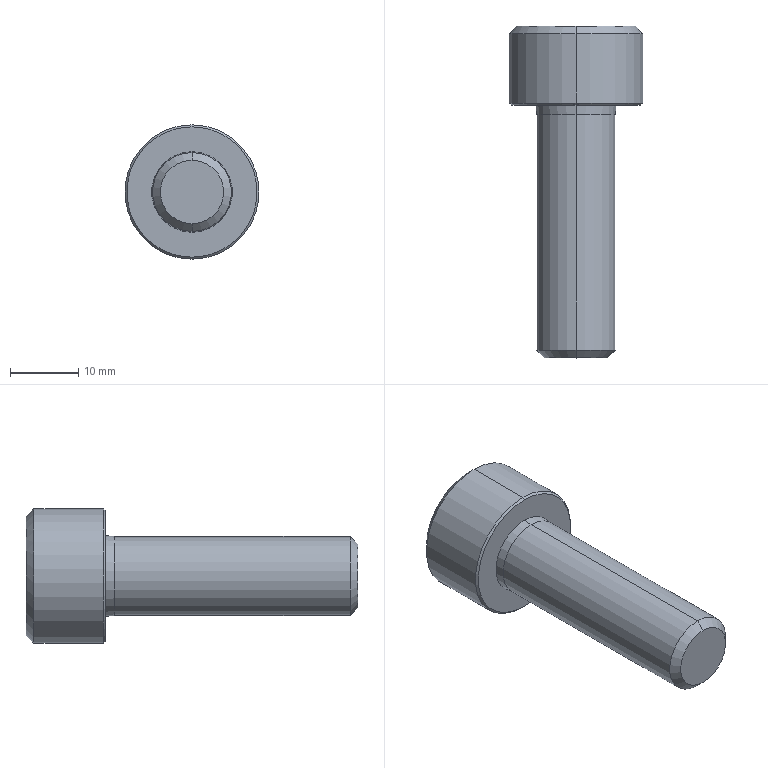Part | SolidWorks | features BaseBody 1 | 1 solid | 35 faces | box 19.615 x 48.462 x 19.615 mm | volume 6797 mm3 | cone 16 | plane 15 | cylinder 4 | commonest cylinder face diameters 11.538 x2 19.615 x2
STEP:
#1=CARTESIAN_POINT('',(-30.446,251.324,298.077));
#2=VERTEX_POINT('',#1);
#3=CARTESIAN_POINT('',(-30.446,251.324,286.538));
#4=VERTEX_POINT('',#3);
#5=CARTESIAN_POINT('',(-30.446,251.324,292.308));
#6=DIRECTION('',(0.,1.,0.));
#7=DIRECTION('',(0.,0.,1.));
#8=AXIS2_PLACEMENT_3D('',#5,#6,#7);
#9=CIRCLE('',#8,5.769);
#10=EDGE_CURVE('',#2,#4,#9,.T.);
#11=ORIENTED_EDGE('',*,*,#10,.T.);
#12=CARTESIAN_POINT('',(-30.446,285.731,286.538));
#13=VERTEX_POINT('',#12);
#14=CARTESIAN_POINT('',(-30.446,250.192,286.538));
#15=DIRECTION('',(0.,1.,0.));
#16=VECTOR('',#15,1000.);
#17=LINE('',#14,#16);
#18=EDGE_CURVE('',#4,#13,#17,.T.);
#19=ORIENTED_EDGE('',*,*,#18,.T.);
#20=CARTESIAN_POINT('',(-30.446,285.731,298.077));
#21=VERTEX_POINT('',#20);
#22=CARTESIAN_POINT('',(-30.446,285.731,292.308));
#23=DIRECTION('',(0.,-1.,0.));
#24=DIRECTION('',(0.,0.,1.));
#25=AXIS2_PLACEMENT_3D('',#22,#23,#24);
#26=CIRCLE('',#25,5.769);
#27=EDGE_CURVE('',#13,#21,#26,.T.);
#28=ORIENTED_EDGE('',*,*,#27,.T.);
#29=CARTESIAN_POINT('',(-30.446,250.192,298.077));
#30=DIRECTION('',(0.,1.,0.));
#31=VECTOR('',#30,1000.);
#32=LINE('',#29,#31);
#33=EDGE_CURVE('',#2,#21,#32,.T.);
#34=ORIENTED_EDGE('',*,*,#33,.F.);
#35=EDGE_LOOP('',(#11,#19,#28,#34));
#36=FACE_OUTER_BOUND('',#35,.T.);
#37=CARTESIAN_POINT('',(-30.446,250.192,292.308));
#38=DIRECTION('',(0.,1.,0.));
#39=DIRECTION('',(0.,0.,1.));
#40=AXIS2_PLACEMENT_3D('',#37,#38,#39);
#41=CYLINDRICAL_SURFACE('',#40,5.769);
#42=ADVANCED_FACE('',(#36),#41,.T.);
#43=CARTESIAN_POINT('',(-30.446,250.192,296.945));
#44=VERTEX_POINT('',#43);
#45=CARTESIAN_POINT('',(-30.446,250.192,287.67));
#46=VERTEX_POINT('',#45);
#47=CARTESIAN_POINT('',(-30.446,250.192,292.308));
#48=DIRECTION('',(0.,1.,0.));
#49=DIRECTION('',(0.,0.,1.));
#50=AXIS2_PLACEMENT_3D('',#47,#48,#49);
#51=CIRCLE('',#50,4.637);
#52=EDGE_CURVE('',#44,#46,#51,.T.);
#53=ORIENTED_EDGE('',*,*,#52,.T.);
#54=CARTESIAN_POINT('',(-30.446,251.324,286.538));
#55=DIRECTION('',(0.,0.7071,-0.7071));
#56=VECTOR('',#55,1000.);
#57=LINE('',#54,#56);
#58=EDGE_CURVE('',#46,#4,#57,.T.);
#59=ORIENTED_EDGE('',*,*,#58,.T.);
#60=ORIENTED_EDGE('',*,*,#10,.F.);
#61=CARTESIAN_POINT('',(-30.446,251.324,298.077));
#62=DIRECTION('',(0.,0.7071,0.7071));
#63=VECTOR('',#62,1000.);
#64=LINE('',#61,#63);
#65=EDGE_CURVE('',#44,#2,#64,.T.);
#66=ORIENTED_EDGE('',*,*,#65,.F.);
#67=EDGE_LOOP('',(#53,#59,#60,#66));
#68=FACE_OUTER_BOUND('',#67,.T.);
#69=CARTESIAN_POINT('',(-30.446,251.324,292.308));
#70=DIRECTION('',(0.,1.,0.));
#71=DIRECTION('',(0.,0.,1.));
#72=AXIS2_PLACEMENT_3D('',#69,#70,#71);
#73=CONICAL_SURFACE('',#72,5.769,0.7854);
#74=ADVANCED_FACE('',(#68),#73,.T.);
#75=ORIENTED_EDGE('',*,*,#27,.F.);
#76=CARTESIAN_POINT('',(-30.446,287.115,286.423));
#77=VERTEX_POINT('',#76);
#78=CARTESIAN_POINT('',(-30.446,287.115,286.423));
#79=DIRECTION('',(0.,0.9965,-0.08305));
#80=VECTOR('',#79,1000.);
#81=LINE('',#78,#80);
#82=EDGE_CURVE('',#13,#77,#81,.T.);
#83=ORIENTED_EDGE('',*,*,#82,.T.);
#84=CARTESIAN_POINT('',(-30.446,287.115,298.192));
#85=VERTEX_POINT('',#84);
#86=CARTESIAN_POINT('',(-30.446,287.115,292.308));
#87=DIRECTION('',(0.,-1.,0.));
#88=DIRECTION('',(0.,0.,1.));
#89=AXIS2_PLACEMENT_3D('',#86,#87,#88);
#90=CIRCLE('',#89,5.885);
#91=EDGE_CURVE('',#77,#85,#90,.T.);
#92=ORIENTED_EDGE('',*,*,#91,.T.);
#93=CARTESIAN_POINT('',(-30.446,287.115,298.192));
#94=DIRECTION('',(0.,0.9965,0.08305));
#95=VECTOR('',#94,1000.);
#96=LINE('',#93,#95);
#97=EDGE_CURVE('',#21,#85,#96,.T.);
#98=ORIENTED_EDGE('',*,*,#97,.F.);
#99=EDGE_LOOP('',(#75,#83,#92,#98));
#100=FACE_OUTER_BOUND('',#99,.T.);
#101=CARTESIAN_POINT('',(-30.446,287.115,292.308));
#102=DIRECTION('',(0.,1.,0.));
#103=DIRECTION('',(0.,0.,1.));
#104=AXIS2_PLACEMENT_3D('',#101,#102,#103);
#105=CONICAL_SURFACE('',#104,5.885,0.08314);
#106=ADVANCED_FACE('',(#100),#105,.T.);
#107=CARTESIAN_POINT('',(-30.446,287.115,301.827));
#108=VERTEX_POINT('',#107);
#109=CARTESIAN_POINT('',(-30.446,287.115,282.788));
#110=VERTEX_POINT('',#109);
#111=CARTESIAN_POINT('',(-30.446,287.115,292.308));
#112=DIRECTION('',(0.,1.,0.));
#113=DIRECTION('',(0.,0.,1.));
#114=AXIS2_PLACEMENT_3D('',#111,#112,#113);
#115=CIRCLE('',#114,9.519);
#116=EDGE_CURVE('',#108,#110,#115,.T.);
#117=ORIENTED_EDGE('',*,*,#116,.T.);
#118=CARTESIAN_POINT('',(-30.446,287.404,282.5));
#119=VERTEX_POINT('',#118);
#120=CARTESIAN_POINT('',(-30.446,287.404,282.5));
#121=DIRECTION('',(0.,0.7071,-0.7071));
#122=VECTOR('',#121,1000.);
#123=LINE('',#120,#122);
#124=EDGE_CURVE('',#110,#119,#123,.T.);
#125=ORIENTED_EDGE('',*,*,#124,.T.);
#126=CARTESIAN_POINT('',(-30.446,287.404,302.115));
#127=VERTEX_POINT('',#126);
#128=CARTESIAN_POINT('',(-30.446,287.404,292.308));
#129=DIRECTION('',(0.,-1.,0.));
#130=DIRECTION('',(0.,0.,1.));
#131=AXIS2_PLACEMENT_3D('',#128,#129,#130);
#132=CIRCLE('',#131,9.808);
#133=EDGE_CURVE('',#119,#127,#132,.T.);
#134=ORIENTED_EDGE('',*,*,#133,.T.);
#135=CARTESIAN_POINT('',(-30.446,287.404,302.115));
#136=DIRECTION('',(0.,0.7071,0.7071));
#137=VECTOR('',#136,1000.);
#138=LINE('',#135,#137);
#139=EDGE_CURVE('',#108,#127,#138,.T.);
#140=ORIENTED_EDGE('',*,*,#139,.F.);
#141=EDGE_LOOP('',(#117,#125,#134,#140));
#142=FACE_OUTER_BOUND('',#141,.T.);
#143=CARTESIAN_POINT('',(-30.446,287.404,292.308));
#144=DIRECTION('',(0.,1.,0.));
#145=DIRECTION('',(0.,0.,1.));
#146=AXIS2_PLACEMENT_3D('',#143,#144,#145);
#147=CONICAL_SURFACE('',#146,9.808,0.7854);
#148=ADVANCED_FACE('',(#142),#147,.T.);
#149=ORIENTED_EDGE('',*,*,#133,.F.);
#150=CARTESIAN_POINT('',(-30.446,297.5,282.5));
#151=VERTEX_POINT('',#150);
#152=CARTESIAN_POINT('',(-30.446,250.192,282.5));
#153=DIRECTION('',(0.,1.,0.));
#154=VECTOR('',#153,1000.);
#155=LINE('',#152,#154);
#156=EDGE_CURVE('',#119,#151,#155,.T.);
#157=ORIENTED_EDGE('',*,*,#156,.T.);
#158=CARTESIAN_POINT('',(-30.446,297.5,302.115));
#159=VERTEX_POINT('',#158);
#160=CARTESIAN_POINT('',(-30.446,297.5,292.308));
#161=DIRECTION('',(0.,-1.,0.));
#162=DIRECTION('',(0.,0.,1.));
#163=AXIS2_PLACEMENT_3D('',#160,#161,#162);
#164=CIRCLE('',#163,9.808);
#165=EDGE_CURVE('',#151,#159,#164,.T.);
#166=ORIENTED_EDGE('',*,*,#165,.T.);
#167=CARTESIAN_POINT('',(-30.446,250.192,302.115));
#168=DIRECTION('',(0.,1.,0.));
#169=VECTOR('',#168,1000.);
#170=LINE('',#167,#169);
#171=EDGE_CURVE('',#127,#159,#170,.T.);
#172=ORIENTED_EDGE('',*,*,#171,.F.);
#173=EDGE_LOOP('',(#149,#157,#166,#172));
#174=FACE_OUTER_BOUND('',#173,.T.);
#175=CARTESIAN_POINT('',(-30.446,250.192,292.308));
#176=DIRECTION('',(0.,1.,0.));
#177=DIRECTION('',(0.,0.,1.));
#178=AXIS2_PLACEMENT_3D('',#175,#176,#177);
#179=CYLINDRICAL_SURFACE('',#178,9.808);
#180=ADVANCED_FACE('',(#174),#179,.T.);
#181=CARTESIAN_POINT('',(-30.446,298.654,283.654));
#182=VERTEX_POINT('',#181);
#183=CARTESIAN_POINT('',(-30.446,298.654,300.962));
#184=VERTEX_POINT('',#183);
#185=CARTESIAN_POINT('',(-30.446,298.654,292.308));
#186=DIRECTION('',(0.,-1.,0.));
#187=DIRECTION('',(0.,0.,-1.));
#188=AXIS2_PLACEMENT_3D('',#185,#186,#187);
#189=CIRCLE('',#188,8.654);
#190=EDGE_CURVE('',#182,#184,#189,.T.);
#191=ORIENTED_EDGE('',*,*,#190,.T.);
#192=CARTESIAN_POINT('',(-30.446,297.5,302.115));
#193=DIRECTION('',(0.,-0.7071,0.7071));
#194=VECTOR('',#193,1000.);
#195=LINE('',#192,#194);
#196=EDGE_CURVE('',#184,#159,#195,.T.);
#197=ORIENTED_EDGE('',*,*,#196,.T.);
#198=ORIENTED_EDGE('',*,*,#165,.F.);
#199=CARTESIAN_POINT('',(-30.446,297.5,282.5));
#200=DIRECTION('',(0.,-0.7071,-0.7071));
#201=VECTOR('',#200,1000.);
#202=LINE('',#199,#201);
#203=EDGE_CURVE('',#182,#151,#202,.T.);
#204=ORIENTED_EDGE('',*,*,#203,.F.);
#205=EDGE_LOOP('',(#191,#197,#198,#204));
#206=FACE_OUTER_BOUND('',#205,.T.);
#207=CARTESIAN_POINT('',(-30.446,297.5,292.308));
#208=DIRECTION('',(0.,-1.,0.));
#209=DIRECTION('',(0.,0.,-1.));
#210=AXIS2_PLACEMENT_3D('',#207,#208,#209);
#211=CONICAL_SURFACE('',#210,9.808,0.7854);
#212=ADVANCED_FACE('',(#206),#211,.T.);
#213=CARTESIAN_POINT('',(-30.446,290.22,292.308));
#214=VERTEX_POINT('',#213);
#215=CARTESIAN_POINT('',(-30.446,292.885,296.923));
#216=VERTEX_POINT('',#215);
#217=CARTESIAN_POINT('',(-30.446,292.885,296.923));
#218=DIRECTION('',(0.,0.5,0.866));
#219=VECTOR('',#218,1000.);
#220=LINE('',#217,#219);
#221=EDGE_CURVE('',#214,#216,#220,.T.);
#222=ORIENTED_EDGE('',*,*,#221,.F.);
#223=CARTESIAN_POINT('',(-30.446,292.885,287.692));
#224=VERTEX_POINT('',#223);
#225=CARTESIAN_POINT('',(-30.446,292.885,287.692));
#226=DIRECTION('',(0.,0.5,-0.866));
#227=VECTOR('',#226,1000.);
#228=LINE('',#225,#227);
#229=EDGE_CURVE('',#214,#224,#228,.T.);
#230=ORIENTED_EDGE('',*,*,#229,.T.);
#231=CARTESIAN_POINT('',(-32.753,292.885,288.311));
#232=VERTEX_POINT('',#231);
#233=CARTESIAN_POINT('',(-30.446,292.885,292.308));
#234=DIRECTION('',(0.,-1.,0.));
#235=DIRECTION('',(0.,0.,1.));
#236=AXIS2_PLACEMENT_3D('',#233,#234,#235);
#237=CIRCLE('',#236,4.615);
#238=EDGE_CURVE('',#232,#224,#237,.T.);
#239=ORIENTED_EDGE('',*,*,#238,.F.);
#240=CARTESIAN_POINT('',(-35.061,292.885,292.308));
#241=VERTEX_POINT('',#240);
#242=CARTESIAN_POINT('',(-30.446,292.885,292.308));
#243=DIRECTION('',(0.,-1.,0.));
#244=DIRECTION('',(0.,0.,1.));
#245=AXIS2_PLACEMENT_3D('',#242,#243,#244);
#246=CIRCLE('',#245,4.615);
#247=EDGE_CURVE('',#241,#232,#246,.T.);
#248=ORIENTED_EDGE('',*,*,#247,.F.);
#249=CARTESIAN_POINT('',(-32.753,292.885,296.305));
#250=VERTEX_POINT('',#249);
#251=CARTESIAN_POINT('',(-30.446,292.885,292.308));
#252=DIRECTION('',(0.,-1.,0.));
#253=DIRECTION('',(0.,0.,1.));
#254=AXIS2_PLACEMENT_3D('',#251,#252,#253);
#255=CIRCLE('',#254,4.615);
#256=EDGE_CURVE('',#250,#241,#255,.T.);
#257=ORIENTED_EDGE('',*,*,#256,.F.);
#258=CARTESIAN_POINT('',(-30.446,292.885,292.308));
#259=DIRECTION('',(0.,-1.,0.));
#260=DIRECTION('',(0.,0.,1.));
#261=AXIS2_PLACEMENT_3D('',#258,#259,#260);
#262=CIRCLE('',#261,4.615);
#263=EDGE_CURVE('',#216,#250,#262,.T.);
#264=ORIENTED_EDGE('',*,*,#263,.F.);
#265=EDGE_LOOP('',(#222,#230,#239,#248,#257,#264));
#266=FACE_OUTER_BOUND('',#265,.T.);
#267=CARTESIAN_POINT('',(-30.446,292.885,292.308));
#268=DIRECTION('',(0.,1.,0.));
#269=DIRECTION('',(0.,0.,1.));
#270=AXIS2_PLACEMENT_3D('',#267,#268,#269);
#271=CONICAL_SURFACE('',#270,4.615,1.047);
#272=ADVANCED_FACE('',(#266),#271,.F.);
#273=ORIENTED_EDGE('',*,*,#18,.F.);
#274=CARTESIAN_POINT('',(-30.446,251.324,292.308));
#275=DIRECTION('',(0.,1.,0.));
#276=DIRECTION('',(0.,0.,1.));
#277=AXIS2_PLACEMENT_3D('',#274,#275,#276);
#278=CIRCLE('',#277,5.769);
#279=EDGE_CURVE('',#4,#2,#278,.T.);
#280=ORIENTED_EDGE('',*,*,#279,.T.);
#281=ORIENTED_EDGE('',*,*,#33,.T.);
#282=CARTESIAN_POINT('',(-30.446,285.731,292.308));
#283=DIRECTION('',(0.,-1.,0.));
#284=DIRECTION('',(0.,0.,1.));
#285=AXIS2_PLACEMENT_3D('',#282,#283,#284);
#286=CIRCLE('',#285,5.769);
#287=EDGE_CURVE('',#21,#13,#286,.T.);
#288=ORIENTED_EDGE('',*,*,#287,.T.);
#289=EDGE_LOOP('',(#273,#280,#281,#288));
#290=FACE_OUTER_BOUND('',#289,.T.);
#291=CARTESIAN_POINT('',(-30.446,250.192,292.308));
#292=DIRECTION('',(0.,1.,0.));
#293=DIRECTION('',(0.,0.,1.));
#294=AXIS2_PLACEMENT_3D('',#291,#292,#293);
#295=CYLINDRICAL_SURFACE('',#294,5.769);
#296=ADVANCED_FACE('',(#290),#295,.T.);
#297=ORIENTED_EDGE('',*,*,#58,.F.);
#298=CARTESIAN_POINT('',(-30.446,250.192,292.308));
#299=DIRECTION('',(0.,1.,0.));
#300=DIRECTION('',(0.,0.,1.));
#301=AXIS2_PLACEMENT_3D('',#298,#299,#300);
#302=CIRCLE('',#301,4.637);
#303=EDGE_CURVE('',#46,#44,#302,.T.);
#304=ORIENTED_EDGE('',*,*,#303,.T.);
#305=ORIENTED_EDGE('',*,*,#65,.T.);
#306=ORIENTED_EDGE('',*,*,#279,.F.);
#307=EDGE_LOOP('',(#297,#304,#305,#306));
#308=FACE_OUTER_BOUND('',#307,.T.);
#309=CARTESIAN_POINT('',(-30.446,251.324,292.308));
#310=DIRECTION('',(0.,1.,0.));
#311=DIRECTION('',(0.,0.,1.));
#312=AXIS2_PLACEMENT_3D('',#309,#310,#311);
#313=CONICAL_SURFACE('',#312,5.769,0.7854);
#314=ADVANCED_FACE('',(#308),#313,.T.);
#315=ORIENTED_EDGE('',*,*,#82,.F.);
#316=ORIENTED_EDGE('',*,*,#287,.F.);
#317=ORIENTED_EDGE('',*,*,#97,.T.);
#318=CARTESIAN_POINT('',(-30.446,287.115,292.308));
#319=DIRECTION('',(0.,-1.,0.));
#320=DIRECTION('',(0.,0.,1.));
#321=AXIS2_PLACEMENT_3D('',#318,#319,#320);
#322=CIRCLE('',#321,5.885);
#323=EDGE_CURVE('',#85,#77,#322,.T.);
#324=ORIENTED_EDGE('',*,*,#323,.T.);
#325=EDGE_LOOP('',(#315,#316,#317,#324));
#326=FACE_OUTER_BOUND('',#325,.T.);
#327=CARTESIAN_POINT('',(-30.446,287.115,292.308));
#328=DIRECTION('',(0.,1.,0.));
#329=DIRECTION('',(0.,0.,1.));
#330=AXIS2_PLACEMENT_3D('',#327,#328,#329);
#331=CONICAL_SURFACE('',#330,5.885,0.08314);
#332=ADVANCED_FACE('',(#326),#331,.T.);
#333=ORIENTED_EDGE('',*,*,#52,.F.);
#334=ORIENTED_EDGE('',*,*,#303,.F.);
#335=EDGE_LOOP('',(#333,#334));
#336=FACE_OUTER_BOUND('',#335,.T.);
#337=CARTESIAN_POINT('',(-35.083,250.192,292.308));
#338=DIRECTION('',(0.,1.,0.));
#339=DIRECTION('',(0.,0.,1.));
#340=AXIS2_PLACEMENT_3D('',#337,#338,#339);
#341=PLANE('',#340);
#342=ADVANCED_FACE('',(#336),#341,.F.);
#343=ORIENTED_EDGE('',*,*,#323,.F.);
#344=ORIENTED_EDGE('',*,*,#91,.F.);
#345=EDGE_LOOP('',(#343,#344));
#346=FACE_BOUND('',#345,.T.);
#347=ORIENTED_EDGE('',*,*,#116,.F.);
#348=CARTESIAN_POINT('',(-30.446,287.115,292.308));
#349=DIRECTION('',(0.,1.,0.));
#350=DIRECTION('',(0.,0.,1.));
#351=AXIS2_PLACEMENT_3D('',#348,#349,#350);
#352=CIRCLE('',#351,9.519);
#353=EDGE_CURVE('',#110,#108,#352,.T.);
#354=ORIENTED_EDGE('',*,*,#353,.F.);
#355=EDGE_LOOP('',(#347,#354));
#356=FACE_OUTER_BOUND('',#355,.T.);
#357=CARTESIAN_POINT('',(-39.965,287.115,292.308));
#358=DIRECTION('',(0.,1.,0.));
#359=DIRECTION('',(0.,0.,1.));
#360=AXIS2_PLACEMENT_3D('',#357,#358,#359);
#361=PLANE('',#360);
#362=ADVANCED_FACE('',(#346,#356),#361,.F.);
#363=ORIENTED_EDGE('',*,*,#124,.F.);
#364=ORIENTED_EDGE('',*,*,#353,.T.);
#365=ORIENTED_EDGE('',*,*,#139,.T.);
#366=CARTESIAN_POINT('',(-30.446,287.404,292.308));
#367=DIRECTION('',(0.,-1.,0.));
#368=DIRECTION('',(0.,0.,1.));
#369=AXIS2_PLACEMENT_3D('',#366,#367,#368);
#370=CIRCLE('',#369,9.808);
#371=EDGE_CURVE('',#127,#119,#370,.T.);
#372=ORIENTED_EDGE('',*,*,#371,.T.);
#373=EDGE_LOOP('',(#363,#364,#365,#372));
#374=FACE_OUTER_BOUND('',#373,.T.);
#375=CARTESIAN_POINT('',(-30.446,287.404,292.308));
#376=DIRECTION('',(0.,1.,0.));
#377=DIRECTION('',(0.,0.,1.));
#378=AXIS2_PLACEMENT_3D('',#375,#376,#377);
#379=CONICAL_SURFACE('',#378,9.808,0.7854);
#380=ADVANCED_FACE('',(#374),#379,.T.);
#381=ORIENTED_EDGE('',*,*,#156,.F.);
#382=ORIENTED_EDGE('',*,*,#371,.F.);
#383=ORIENTED_EDGE('',*,*,#171,.T.);
#384=CARTESIAN_POINT('',(-30.446,297.5,292.308));
#385=DIRECTION('',(0.,-1.,0.));
#386=DIRECTION('',(0.,0.,1.));
#387=AXIS2_PLACEMENT_3D('',#384,#385,#386);
#388=CIRCLE('',#387,9.808);
#389=EDGE_CURVE('',#159,#151,#388,.T.);
#390=ORIENTED_EDGE('',*,*,#389,.T.);
#391=EDGE_LOOP('',(#381,#382,#383,#390));
#392=FACE_OUTER_BOUND('',#391,.T.);
#393=CARTESIAN_POINT('',(-30.446,250.192,292.308));
#394=DIRECTION('',(0.,1.,0.));
#395=DIRECTION('',(0.,0.,1.));
#396=AXIS2_PLACEMENT_3D('',#393,#394,#395);
#397=CYLINDRICAL_SURFACE('',#396,9.808);
#398=ADVANCED_FACE('',(#392),#397,.T.);
#399=ORIENTED_EDGE('',*,*,#196,.F.);
#400=CARTESIAN_POINT('',(-30.446,298.654,292.308));
#401=DIRECTION('',(0.,-1.,0.));
#402=DIRECTION('',(0.,0.,-1.));
#403=AXIS2_PLACEMENT_3D('',#400,#401,#402);
#404=CIRCLE('',#403,8.654);
#405=EDGE_CURVE('',#184,#182,#404,.T.);
#406=ORIENTED_EDGE('',*,*,#405,.T.);
#407=ORIENTED_EDGE('',*,*,#203,.T.);
#408=ORIENTED_EDGE('',*,*,#389,.F.);
#409=EDGE_LOOP('',(#399,#406,#407,#408));
#410=FACE_OUTER_BOUND('',#409,.T.);
#411=CARTESIAN_POINT('',(-30.446,297.5,292.308));
#412=DIRECTION('',(0.,-1.,0.));
#413=DIRECTION('',(0.,0.,-1.));
#414=AXIS2_PLACEMENT_3D('',#411,#412,#413);
#415=CONICAL_SURFACE('',#414,9.808,0.7854);
#416=ADVANCED_FACE('',(#410),#415,.T.);
#417=CARTESIAN_POINT('',(-25.83,298.654,289.643));
#418=VERTEX_POINT('',#417);
#419=CARTESIAN_POINT('',(-30.446,298.654,286.978));
#420=VERTEX_POINT('',#419);
#421=CARTESIAN_POINT('',(-30.446,298.654,292.308));
#422=DIRECTION('',(0.,1.,0.));
#423=DIRECTION('',(0.,0.,1.));
#424=AXIS2_PLACEMENT_3D('',#421,#422,#423);
#425=CIRCLE('',#424,5.329);
#426=EDGE_CURVE('',#418,#420,#425,.T.);
#427=ORIENTED_EDGE('',*,*,#426,.F.);
#428=CARTESIAN_POINT('',(-25.83,298.654,294.972));
#429=VERTEX_POINT('',#428);
#430=CARTESIAN_POINT('',(-30.446,298.654,292.308));
#431=DIRECTION('',(0.,1.,0.));
#432=DIRECTION('',(0.,0.,1.));
#433=AXIS2_PLACEMENT_3D('',#430,#431,#432);
#434=CIRCLE('',#433,5.329);
#435=EDGE_CURVE('',#429,#418,#434,.T.);
#436=ORIENTED_EDGE('',*,*,#435,.F.);
#437=CARTESIAN_POINT('',(-30.446,298.654,297.637));
#438=VERTEX_POINT('',#437);
#439=CARTESIAN_POINT('',(-30.446,298.654,292.308));
#440=DIRECTION('',(0.,1.,0.));
#441=DIRECTION('',(0.,0.,1.));
#442=AXIS2_PLACEMENT_3D('',#439,#440,#441);
#443=CIRCLE('',#442,5.329);
#444=EDGE_CURVE('',#438,#429,#443,.T.);
#445=ORIENTED_EDGE('',*,*,#444,.F.);
#446=CARTESIAN_POINT('',(-35.061,298.654,294.972));
#447=VERTEX_POINT('',#446);
#448=CARTESIAN_POINT('',(-30.446,298.654,292.308));
#449=DIRECTION('',(0.,1.,0.));
#450=DIRECTION('',(0.,0.,1.));
#451=AXIS2_PLACEMENT_3D('',#448,#449,#450);
#452=CIRCLE('',#451,5.329);
#453=EDGE_CURVE('',#447,#438,#452,.T.);
#454=ORIENTED_EDGE('',*,*,#453,.F.);
#455=CARTESIAN_POINT('',(-35.061,298.654,289.643));
#456=VERTEX_POINT('',#455);
#457=CARTESIAN_POINT('',(-30.446,298.654,292.308));
#458=DIRECTION('',(0.,1.,0.));
#459=DIRECTION('',(0.,0.,1.));
#460=AXIS2_PLACEMENT_3D('',#457,#458,#459);
#461=CIRCLE('',#460,5.329);
#462=EDGE_CURVE('',#456,#447,#461,.T.);
#463=ORIENTED_EDGE('',*,*,#462,.F.);
#464=CARTESIAN_POINT('',(-30.446,298.654,292.308));
#465=DIRECTION('',(0.,1.,0.));
#466=DIRECTION('',(0.,0.,1.));
#467=AXIS2_PLACEMENT_3D('',#464,#465,#466);
#468=CIRCLE('',#467,5.329);
#469=EDGE_CURVE('',#420,#456,#468,.T.);
#470=ORIENTED_EDGE('',*,*,#469,.F.);
#471=EDGE_LOOP('',(#427,#436,#445,#454,#463,#470));
#472=FACE_BOUND('',#471,.T.);
#473=ORIENTED_EDGE('',*,*,#190,.F.);
#474=ORIENTED_EDGE('',*,*,#405,.F.);
#475=EDGE_LOOP('',(#473,#474));
#476=FACE_OUTER_BOUND('',#475,.T.);
#477=CARTESIAN_POINT('',(-35.775,298.654,292.308));
#478=DIRECTION('',(0.,-1.,0.));
#479=DIRECTION('',(0.,0.,-1.));
#480=AXIS2_PLACEMENT_3D('',#477,#478,#479);
#481=PLANE('',#480);
#482=ADVANCED_FACE('',(#472,#476),#481,.F.);
#483=CARTESIAN_POINT('',(-30.446,298.654,286.978));
#484=CARTESIAN_POINT('',(-30.806,298.446,287.187));
#485=CARTESIAN_POINT('',(-31.175,298.269,287.399));
#486=CARTESIAN_POINT('',(-31.748,298.079,287.73));
#487=CARTESIAN_POINT('',(-31.942,298.029,287.842));
#488=CARTESIAN_POINT('',(-32.339,297.959,288.071));
#489=CARTESIAN_POINT('',(-32.544,297.94,288.189));
#490=CARTESIAN_POINT('',(-33.148,297.939,288.538));
#491=CARTESIAN_POINT('',(-33.544,298.009,288.767));
#492=CARTESIAN_POINT('',(-34.325,298.265,289.218));
#493=CARTESIAN_POINT('',(-34.698,298.444,289.434));
#494=CARTESIAN_POINT('',(-35.061,298.654,289.643));
#495=B_SPLINE_CURVE_WITH_KNOTS('',3,(#483,#484,#485,#486,#487,#488,#489,#490,#491,#492,#493,#494),.UNSPECIFIED.,.F.,.F.,(4,2,2,2,2,4),(0.,0.001376,0.002064,0.002753,0.004129,0.005505),.UNSPECIFIED.);
#496=EDGE_CURVE('',#420,#456,#495,.T.);
#497=ORIENTED_EDGE('',*,*,#496,.F.);
#498=ORIENTED_EDGE('',*,*,#469,.T.);
#499=EDGE_LOOP('',(#497,#498));
#500=FACE_OUTER_BOUND('',#499,.T.);
#501=CARTESIAN_POINT('',(-30.446,298.654,292.308));
#502=DIRECTION('',(0.,1.,0.));
#503=DIRECTION('',(0.,0.,1.));
#504=AXIS2_PLACEMENT_3D('',#501,#502,#503);
#505=CONICAL_SURFACE('',#504,5.329,0.7854);
#506=ADVANCED_FACE('',(#500),#505,.F.);
#507=CARTESIAN_POINT('',(-25.83,298.654,289.643));
#508=CARTESIAN_POINT('',(-26.191,298.446,289.435));
#509=CARTESIAN_POINT('',(-26.56,298.269,289.222));
#510=CARTESIAN_POINT('',(-27.133,298.079,288.891));
#511=CARTESIAN_POINT('',(-27.327,298.029,288.779));
#512=CARTESIAN_POINT('',(-27.724,297.959,288.55));
#513=CARTESIAN_POINT('',(-27.928,297.94,288.432));
#514=CARTESIAN_POINT('',(-28.533,297.939,288.083));
#515=CARTESIAN_POINT('',(-28.929,298.009,287.854));
#516=CARTESIAN_POINT('',(-29.71,298.265,287.403));
#517=CARTESIAN_POINT('',(-30.083,298.444,287.188));
#518=CARTESIAN_POINT('',(-30.446,298.654,286.978));
#519=B_SPLINE_CURVE_WITH_KNOTS('',3,(#507,#508,#509,#510,#511,#512,#513,#514,#515,#516,#517,#518),.UNSPECIFIED.,.F.,.F.,(4,2,2,2,2,4),(0.,0.001376,0.002064,0.002753,0.004129,0.005505),.UNSPECIFIED.);
#520=EDGE_CURVE('',#418,#420,#519,.T.);
#521=ORIENTED_EDGE('',*,*,#520,.F.);
#522=ORIENTED_EDGE('',*,*,#426,.T.);
#523=EDGE_LOOP('',(#521,#522));
#524=FACE_OUTER_BOUND('',#523,.T.);
#525=CARTESIAN_POINT('',(-30.446,298.654,292.308));
#526=DIRECTION('',(0.,1.,0.));
#527=DIRECTION('',(0.,0.,1.));
#528=AXIS2_PLACEMENT_3D('',#525,#526,#527);
#529=CONICAL_SURFACE('',#528,5.329,0.7854);
#530=ADVANCED_FACE('',(#524),#529,.F.);
#531=CARTESIAN_POINT('',(-25.83,298.654,294.972));
#532=CARTESIAN_POINT('',(-25.83,298.446,294.556));
#533=CARTESIAN_POINT('',(-25.83,298.269,294.13));
#534=CARTESIAN_POINT('',(-25.83,298.079,293.469));
#535=CARTESIAN_POINT('',(-25.83,298.029,293.244));
#536=CARTESIAN_POINT('',(-25.83,297.959,292.786));
#537=CARTESIAN_POINT('',(-25.83,297.94,292.55));
#538=CARTESIAN_POINT('',(-25.83,297.939,291.852));
#539=CARTESIAN_POINT('',(-25.83,298.009,291.395));
#540=CARTESIAN_POINT('',(-25.83,298.265,290.493));
#541=CARTESIAN_POINT('',(-25.83,298.444,290.062));
#542=CARTESIAN_POINT('',(-25.83,298.654,289.643));
#543=B_SPLINE_CURVE_WITH_KNOTS('',3,(#531,#532,#533,#534,#535,#536,#537,#538,#539,#540,#541,#542),.UNSPECIFIED.,.F.,.F.,(4,2,2,2,2,4),(0.,0.001376,0.002064,0.002753,0.004129,0.005505),.UNSPECIFIED.);
#544=EDGE_CURVE('',#429,#418,#543,.T.);
#545=ORIENTED_EDGE('',*,*,#544,.F.);
#546=ORIENTED_EDGE('',*,*,#435,.T.);
#547=EDGE_LOOP('',(#545,#546));
#548=FACE_OUTER_BOUND('',#547,.T.);
#549=CARTESIAN_POINT('',(-30.446,298.654,292.308));
#550=DIRECTION('',(0.,1.,0.));
#551=DIRECTION('',(0.,0.,1.));
#552=AXIS2_PLACEMENT_3D('',#549,#550,#551);
#553=CONICAL_SURFACE('',#552,5.329,0.7854);
#554=ADVANCED_FACE('',(#548),#553,.F.);
#555=CARTESIAN_POINT('',(-30.446,298.654,297.637));
#556=CARTESIAN_POINT('',(-30.085,298.446,297.429));
#557=CARTESIAN_POINT('',(-29.716,298.269,297.216));
#558=CARTESIAN_POINT('',(-29.144,298.079,296.885));
#559=CARTESIAN_POINT('',(-28.949,298.029,296.773));
#560=CARTESIAN_POINT('',(-28.552,297.959,296.544));
#561=CARTESIAN_POINT('',(-28.348,297.94,296.426));
#562=CARTESIAN_POINT('',(-27.744,297.939,296.077));
#563=CARTESIAN_POINT('',(-27.348,298.009,295.848));
#564=CARTESIAN_POINT('',(-26.567,298.265,295.397));
#565=CARTESIAN_POINT('',(-26.193,298.444,295.182));
#566=CARTESIAN_POINT('',(-25.83,298.654,294.972));
#567=B_SPLINE_CURVE_WITH_KNOTS('',3,(#555,#556,#557,#558,#559,#560,#561,#562,#563,#564,#565,#566),.UNSPECIFIED.,.F.,.F.,(4,2,2,2,2,4),(0.,0.001376,0.002064,0.002753,0.004129,0.005505),.UNSPECIFIED.);
#568=EDGE_CURVE('',#438,#429,#567,.T.);
#569=ORIENTED_EDGE('',*,*,#568,.F.);
#570=ORIENTED_EDGE('',*,*,#444,.T.);
#571=EDGE_LOOP('',(#569,#570));
#572=FACE_OUTER_BOUND('',#571,.T.);
#573=CARTESIAN_POINT('',(-30.446,298.654,292.308));
#574=DIRECTION('',(0.,1.,0.));
#575=DIRECTION('',(0.,0.,1.));
#576=AXIS2_PLACEMENT_3D('',#573,#574,#575);
#577=CONICAL_SURFACE('',#576,5.329,0.7854);
#578=ADVANCED_FACE('',(#572),#577,.F.);
#579=CARTESIAN_POINT('',(-35.061,298.654,294.972));
#580=CARTESIAN_POINT('',(-34.701,298.446,295.181));
#581=CARTESIAN_POINT('',(-34.332,298.269,295.393));
#582=CARTESIAN_POINT('',(-33.759,298.079,295.724));
#583=CARTESIAN_POINT('',(-33.565,298.029,295.836));
#584=CARTESIAN_POINT('',(-33.168,297.959,296.066));
#585=CARTESIAN_POINT('',(-32.963,297.94,296.184));
#586=CARTESIAN_POINT('',(-32.359,297.939,296.532));
#587=CARTESIAN_POINT('',(-31.963,298.009,296.761));
#588=CARTESIAN_POINT('',(-31.182,298.265,297.212));
#589=CARTESIAN_POINT('',(-30.809,298.444,297.428));
#590=CARTESIAN_POINT('',(-30.446,298.654,297.637));
#591=B_SPLINE_CURVE_WITH_KNOTS('',3,(#579,#580,#581,#582,#583,#584,#585,#586,#587,#588,#589,#590),.UNSPECIFIED.,.F.,.F.,(4,2,2,2,2,4),(0.,0.001376,0.002064,0.002753,0.004129,0.005505),.UNSPECIFIED.);
#592=EDGE_CURVE('',#447,#438,#591,.T.);
#593=ORIENTED_EDGE('',*,*,#592,.F.);
#594=ORIENTED_EDGE('',*,*,#453,.T.);
#595=EDGE_LOOP('',(#593,#594));
#596=FACE_OUTER_BOUND('',#595,.T.);
#597=CARTESIAN_POINT('',(-30.446,298.654,292.308));
#598=DIRECTION('',(0.,1.,0.));
#599=DIRECTION('',(0.,0.,1.));
#600=AXIS2_PLACEMENT_3D('',#597,#598,#599);
#601=CONICAL_SURFACE('',#600,5.329,0.7854);
#602=ADVANCED_FACE('',(#596),#601,.F.);
#603=CARTESIAN_POINT('',(-35.061,298.654,289.643));
#604=CARTESIAN_POINT('',(-35.061,298.446,290.059));
#605=CARTESIAN_POINT('',(-35.061,298.269,290.485));
#606=CARTESIAN_POINT('',(-35.061,298.079,291.147));
#607=CARTESIAN_POINT('',(-35.061,298.029,291.371));
#608=CARTESIAN_POINT('',(-35.061,297.959,291.829));
#609=CARTESIAN_POINT('',(-35.061,297.94,292.065));
#610=CARTESIAN_POINT('',(-35.061,297.939,292.763));
#611=CARTESIAN_POINT('',(-35.061,298.009,293.22));
#612=CARTESIAN_POINT('',(-35.061,298.265,294.122));
#613=CARTESIAN_POINT('',(-35.061,298.444,294.554));
#614=CARTESIAN_POINT('',(-35.061,298.654,294.972));
#615=B_SPLINE_CURVE_WITH_KNOTS('',3,(#603,#604,#605,#606,#607,#608,#609,#610,#611,#612,#613,#614),.UNSPECIFIED.,.F.,.F.,(4,2,2,2,2,4),(0.,0.001376,0.002064,0.002753,0.004129,0.005505),.UNSPECIFIED.);
#616=EDGE_CURVE('',#456,#447,#615,.T.);
#617=ORIENTED_EDGE('',*,*,#616,.F.);
#618=ORIENTED_EDGE('',*,*,#462,.T.);
#619=EDGE_LOOP('',(#617,#618));
#620=FACE_OUTER_BOUND('',#619,.T.);
#621=CARTESIAN_POINT('',(-30.446,298.654,292.308));
#622=DIRECTION('',(0.,1.,0.));
#623=DIRECTION('',(0.,0.,1.));
#624=AXIS2_PLACEMENT_3D('',#621,#622,#623);
#625=CONICAL_SURFACE('',#624,5.329,0.7854);
#626=ADVANCED_FACE('',(#620),#625,.F.);
#627=CARTESIAN_POINT('',(-35.061,292.885,289.643));
#628=VERTEX_POINT('',#627);
#629=CARTESIAN_POINT('',(-35.061,292.885,289.643));
#630=DIRECTION('',(0.,1.,0.));
#631=VECTOR('',#630,1000.);
#632=LINE('',#629,#631);
#633=EDGE_CURVE('',#628,#456,#632,.T.);
#634=ORIENTED_EDGE('',*,*,#633,.F.);
#635=CARTESIAN_POINT('',(-30.446,292.885,286.978));
#636=DIRECTION('',(-0.866,0.,0.5));
#637=VECTOR('',#636,1000.);
#638=LINE('',#635,#637);
#639=EDGE_CURVE('',#232,#628,#638,.T.);
#640=ORIENTED_EDGE('',*,*,#639,.F.);
#641=CARTESIAN_POINT('',(-30.446,292.885,286.978));
#642=VERTEX_POINT('',#641);
#643=CARTESIAN_POINT('',(-30.446,292.885,286.978));
#644=DIRECTION('',(-0.866,0.,0.5));
#645=VECTOR('',#644,1000.);
#646=LINE('',#643,#645);
#647=EDGE_CURVE('',#642,#232,#646,.T.);
#648=ORIENTED_EDGE('',*,*,#647,.F.);
#649=CARTESIAN_POINT('',(-30.446,292.885,286.978));
#650=DIRECTION('',(0.,-1.,0.));
#651=VECTOR('',#650,1000.);
#652=LINE('',#649,#651);
#653=EDGE_CURVE('',#420,#642,#652,.T.);
#654=ORIENTED_EDGE('',*,*,#653,.F.);
#655=ORIENTED_EDGE('',*,*,#496,.T.);
#656=EDGE_LOOP('',(#634,#640,#648,#654,#655));
#657=FACE_OUTER_BOUND('',#656,.T.);
#658=CARTESIAN_POINT('',(-30.446,292.885,286.978));
#659=DIRECTION('',(-0.5,0.,-0.866));
#660=DIRECTION('',(-0.866,0.,0.5));
#661=AXIS2_PLACEMENT_3D('',#658,#659,#660);
#662=PLANE('',#661);
#663=ADVANCED_FACE('',(#657),#662,.F.);
#664=ORIENTED_EDGE('',*,*,#653,.T.);
#665=CARTESIAN_POINT('',(-28.138,292.885,288.311));
#666=VERTEX_POINT('',#665);
#667=CARTESIAN_POINT('',(-25.83,292.885,289.643));
#668=DIRECTION('',(-0.866,0.,-0.5));
#669=VECTOR('',#668,1000.);
#670=LINE('',#667,#669);
#671=EDGE_CURVE('',#666,#642,#670,.T.);
#672=ORIENTED_EDGE('',*,*,#671,.F.);
#673=CARTESIAN_POINT('',(-25.83,292.885,289.643));
#674=VERTEX_POINT('',#673);
#675=CARTESIAN_POINT('',(-25.83,292.885,289.643));
#676=DIRECTION('',(-0.866,0.,-0.5));
#677=VECTOR('',#676,1000.);
#678=LINE('',#675,#677);
#679=EDGE_CURVE('',#674,#666,#678,.T.);
#680=ORIENTED_EDGE('',*,*,#679,.F.);
#681=CARTESIAN_POINT('',(-25.83,292.885,289.643));
#682=DIRECTION('',(0.,-1.,0.));
#683=VECTOR('',#682,1000.);
#684=LINE('',#681,#683);
#685=EDGE_CURVE('',#418,#674,#684,.T.);
#686=ORIENTED_EDGE('',*,*,#685,.F.);
#687=ORIENTED_EDGE('',*,*,#520,.T.);
#688=EDGE_LOOP('',(#664,#672,#680,#686,#687));
#689=FACE_OUTER_BOUND('',#688,.T.);
#690=CARTESIAN_POINT('',(-25.83,292.885,289.643));
#691=DIRECTION('',(0.5,0.,-0.866));
#692=DIRECTION('',(-0.866,0.,-0.5));
#693=AXIS2_PLACEMENT_3D('',#690,#691,#692);
#694=PLANE('',#693);
#695=ADVANCED_FACE('',(#689),#694,.F.);
#696=ORIENTED_EDGE('',*,*,#685,.T.);
#697=CARTESIAN_POINT('',(-25.83,292.885,292.308));
#698=VERTEX_POINT('',#697);
#699=CARTESIAN_POINT('',(-25.83,292.885,294.972));
#700=DIRECTION('',(0.,0.,-1.));
#701=VECTOR('',#700,1000.);
#702=LINE('',#699,#701);
#703=EDGE_CURVE('',#698,#674,#702,.T.);
#704=ORIENTED_EDGE('',*,*,#703,.F.);
#705=CARTESIAN_POINT('',(-25.83,292.885,294.972));
#706=VERTEX_POINT('',#705);
#707=CARTESIAN_POINT('',(-25.83,292.885,294.972));
#708=DIRECTION('',(0.,0.,-1.));
#709=VECTOR('',#708,1000.);
#710=LINE('',#707,#709);
#711=EDGE_CURVE('',#706,#698,#710,.T.);
#712=ORIENTED_EDGE('',*,*,#711,.F.);
#713=CARTESIAN_POINT('',(-25.83,292.885,294.972));
#714=DIRECTION('',(0.,-1.,0.));
#715=VECTOR('',#714,1000.);
#716=LINE('',#713,#715);
#717=EDGE_CURVE('',#429,#706,#716,.T.);
#718=ORIENTED_EDGE('',*,*,#717,.F.);
#719=ORIENTED_EDGE('',*,*,#544,.T.);
#720=EDGE_LOOP('',(#696,#704,#712,#718,#719));
#721=FACE_OUTER_BOUND('',#720,.T.);
#722=CARTESIAN_POINT('',(-25.83,292.885,294.972));
#723=DIRECTION('',(1.,0.,0.));
#724=DIRECTION('',(0.,0.,-1.));
#725=AXIS2_PLACEMENT_3D('',#722,#723,#724);
#726=PLANE('',#725);
#727=ADVANCED_FACE('',(#721),#726,.F.);
#728=ORIENTED_EDGE('',*,*,#717,.T.);
#729=CARTESIAN_POINT('',(-28.138,292.885,296.305));
#730=VERTEX_POINT('',#729);
#731=CARTESIAN_POINT('',(-30.446,292.885,297.637));
#732=DIRECTION('',(0.866,0.,-0.5));
#733=VECTOR('',#732,1000.);
#734=LINE('',#731,#733);
#735=EDGE_CURVE('',#730,#706,#734,.T.);
#736=ORIENTED_EDGE('',*,*,#735,.F.);
#737=CARTESIAN_POINT('',(-30.446,292.885,297.637));
#738=VERTEX_POINT('',#737);
#739=CARTESIAN_POINT('',(-30.446,292.885,297.637));
#740=DIRECTION('',(0.866,0.,-0.5));
#741=VECTOR('',#740,1000.);
#742=LINE('',#739,#741);
#743=EDGE_CURVE('',#738,#730,#742,.T.);
#744=ORIENTED_EDGE('',*,*,#743,.F.);
#745=CARTESIAN_POINT('',(-30.446,292.885,297.637));
#746=DIRECTION('',(0.,-1.,0.));
#747=VECTOR('',#746,1000.);
#748=LINE('',#745,#747);
#749=EDGE_CURVE('',#438,#738,#748,.T.);
#750=ORIENTED_EDGE('',*,*,#749,.F.);
#751=ORIENTED_EDGE('',*,*,#568,.T.);
#752=EDGE_LOOP('',(#728,#736,#744,#750,#751));
#753=FACE_OUTER_BOUND('',#752,.T.);
#754=CARTESIAN_POINT('',(-30.446,292.885,297.637));
#755=DIRECTION('',(0.5,0.,0.866));
#756=DIRECTION('',(0.866,0.,-0.5));
#757=AXIS2_PLACEMENT_3D('',#754,#755,#756);
#758=PLANE('',#757);
#759=ADVANCED_FACE('',(#753),#758,.F.);
#760=ORIENTED_EDGE('',*,*,#749,.T.);
#761=CARTESIAN_POINT('',(-35.061,292.885,294.972));
#762=DIRECTION('',(0.866,0.,0.5));
#763=VECTOR('',#762,1000.);
#764=LINE('',#761,#763);
#765=EDGE_CURVE('',#250,#738,#764,.T.);
#766=ORIENTED_EDGE('',*,*,#765,.F.);
#767=CARTESIAN_POINT('',(-35.061,292.885,294.972));
#768=VERTEX_POINT('',#767);
#769=CARTESIAN_POINT('',(-35.061,292.885,294.972));
#770=DIRECTION('',(0.866,0.,0.5));
#771=VECTOR('',#770,1000.);
#772=LINE('',#769,#771);
#773=EDGE_CURVE('',#768,#250,#772,.T.);
#774=ORIENTED_EDGE('',*,*,#773,.F.);
#775=CARTESIAN_POINT('',(-35.061,292.885,294.972));
#776=DIRECTION('',(0.,-1.,0.));
#777=VECTOR('',#776,1000.);
#778=LINE('',#775,#777);
#779=EDGE_CURVE('',#447,#768,#778,.T.);
#780=ORIENTED_EDGE('',*,*,#779,.F.);
#781=ORIENTED_EDGE('',*,*,#592,.T.);
#782=EDGE_LOOP('',(#760,#766,#774,#780,#781));
#783=FACE_OUTER_BOUND('',#782,.T.);
#784=CARTESIAN_POINT('',(-35.061,292.885,294.972));
#785=DIRECTION('',(-0.5,0.,0.866));
#786=DIRECTION('',(0.866,0.,0.5));
#787=AXIS2_PLACEMENT_3D('',#784,#785,#786);
#788=PLANE('',#787);
#789=ADVANCED_FACE('',(#783),#788,.F.);
#790=ORIENTED_EDGE('',*,*,#779,.T.);
#791=CARTESIAN_POINT('',(-35.061,292.885,289.643));
#792=DIRECTION('',(0.,0.,1.));
#793=VECTOR('',#792,1000.);
#794=LINE('',#791,#793);
#795=EDGE_CURVE('',#241,#768,#794,.T.);
#796=ORIENTED_EDGE('',*,*,#795,.F.);
#797=CARTESIAN_POINT('',(-35.061,292.885,289.643));
#798=DIRECTION('',(0.,0.,1.));
#799=VECTOR('',#798,1000.);
#800=LINE('',#797,#799);
#801=EDGE_CURVE('',#628,#241,#800,.T.);
#802=ORIENTED_EDGE('',*,*,#801,.F.);
#803=ORIENTED_EDGE('',*,*,#633,.T.);
#804=ORIENTED_EDGE('',*,*,#616,.T.);
#805=EDGE_LOOP('',(#790,#796,#802,#803,#804));
#806=FACE_OUTER_BOUND('',#805,.T.);
#807=CARTESIAN_POINT('',(-35.061,292.885,289.643));
#808=DIRECTION('',(-1.,0.,0.));
#809=DIRECTION('',(0.,0.,1.));
#810=AXIS2_PLACEMENT_3D('',#807,#808,#809);
#811=PLANE('',#810);
#812=ADVANCED_FACE('',(#806),#811,.F.);
#813=ORIENTED_EDGE('',*,*,#247,.T.);
#814=ORIENTED_EDGE('',*,*,#639,.T.);
#815=ORIENTED_EDGE('',*,*,#801,.T.);
#816=EDGE_LOOP('',(#813,#814,#815));
#817=FACE_OUTER_BOUND('',#816,.T.);
#818=CARTESIAN_POINT('',(-30.446,292.885,292.308));
#819=DIRECTION('',(0.,1.,0.));
#820=DIRECTION('',(0.,0.,1.));
#821=AXIS2_PLACEMENT_3D('',#818,#819,#820);
#822=PLANE('',#821);
#823=ADVANCED_FACE('',(#817),#822,.T.);
#824=ORIENTED_EDGE('',*,*,#238,.T.);
#825=CARTESIAN_POINT('',(-30.446,292.885,292.308));
#826=DIRECTION('',(0.,-1.,0.));
#827=DIRECTION('',(0.,0.,1.));
#828=AXIS2_PLACEMENT_3D('',#825,#826,#827);
#829=CIRCLE('',#828,4.615);
#830=EDGE_CURVE('',#224,#666,#829,.T.);
#831=ORIENTED_EDGE('',*,*,#830,.T.);
#832=ORIENTED_EDGE('',*,*,#671,.T.);
#833=ORIENTED_EDGE('',*,*,#647,.T.);
#834=EDGE_LOOP('',(#824,#831,#832,#833));
#835=FACE_OUTER_BOUND('',#834,.T.);
#836=CARTESIAN_POINT('',(-30.446,292.885,292.308));
#837=DIRECTION('',(0.,1.,0.));
#838=DIRECTION('',(0.,0.,1.));
#839=AXIS2_PLACEMENT_3D('',#836,#837,#838);
#840=PLANE('',#839);
#841=ADVANCED_FACE('',(#835),#840,.T.);
#842=CARTESIAN_POINT('',(-30.446,292.885,292.308));
#843=DIRECTION('',(0.,-1.,0.));
#844=DIRECTION('',(0.,0.,1.));
#845=AXIS2_PLACEMENT_3D('',#842,#843,#844);
#846=CIRCLE('',#845,4.615);
#847=EDGE_CURVE('',#666,#698,#846,.T.);
#848=ORIENTED_EDGE('',*,*,#847,.T.);
#849=ORIENTED_EDGE('',*,*,#703,.T.);
#850=ORIENTED_EDGE('',*,*,#679,.T.);
#851=EDGE_LOOP('',(#848,#849,#850));
#852=FACE_OUTER_BOUND('',#851,.T.);
#853=CARTESIAN_POINT('',(-30.446,292.885,292.308));
#854=DIRECTION('',(0.,1.,0.));
#855=DIRECTION('',(0.,0.,1.));
#856=AXIS2_PLACEMENT_3D('',#853,#854,#855);
#857=PLANE('',#856);
#858=ADVANCED_FACE('',(#852),#857,.T.);
#859=CARTESIAN_POINT('',(-30.446,292.885,292.308));
#860=DIRECTION('',(0.,-1.,0.));
#861=DIRECTION('',(0.,0.,1.));
#862=AXIS2_PLACEMENT_3D('',#859,#860,#861);
#863=CIRCLE('',#862,4.615);
#864=EDGE_CURVE('',#698,#730,#863,.T.);
#865=ORIENTED_EDGE('',*,*,#864,.T.);
#866=ORIENTED_EDGE('',*,*,#735,.T.);
#867=ORIENTED_EDGE('',*,*,#711,.T.);
#868=EDGE_LOOP('',(#865,#866,#867));
#869=FACE_OUTER_BOUND('',#868,.T.);
#870=CARTESIAN_POINT('',(-30.446,292.885,292.308));
#871=DIRECTION('',(0.,1.,0.));
#872=DIRECTION('',(0.,0.,1.));
#873=AXIS2_PLACEMENT_3D('',#870,#871,#872);
#874=PLANE('',#873);
#875=ADVANCED_FACE('',(#869),#874,.T.);
#876=CARTESIAN_POINT('',(-30.446,292.885,292.308));
#877=DIRECTION('',(0.,-1.,0.));
#878=DIRECTION('',(0.,0.,1.));
#879=AXIS2_PLACEMENT_3D('',#876,#877,#878);
#880=CIRCLE('',#879,4.615);
#881=EDGE_CURVE('',#730,#216,#880,.T.);
#882=ORIENTED_EDGE('',*,*,#881,.T.);
#883=ORIENTED_EDGE('',*,*,#263,.T.);
#884=ORIENTED_EDGE('',*,*,#765,.T.);
#885=ORIENTED_EDGE('',*,*,#743,.T.);
#886=EDGE_LOOP('',(#882,#883,#884,#885));
#887=FACE_OUTER_BOUND('',#886,.T.);
#888=CARTESIAN_POINT('',(-30.446,292.885,292.308));
#889=DIRECTION('',(0.,1.,0.));
#890=DIRECTION('',(0.,0.,1.));
#891=AXIS2_PLACEMENT_3D('',#888,#889,#890);
#892=PLANE('',#891);
#893=ADVANCED_FACE('',(#887),#892,.T.);
#894=ORIENTED_EDGE('',*,*,#256,.T.);
#895=ORIENTED_EDGE('',*,*,#795,.T.);
#896=ORIENTED_EDGE('',*,*,#773,.T.);
#897=EDGE_LOOP('',(#894,#895,#896));
#898=FACE_OUTER_BOUND('',#897,.T.);
#899=CARTESIAN_POINT('',(-30.446,292.885,292.308));
#900=DIRECTION('',(0.,1.,0.));
#901=DIRECTION('',(0.,0.,1.));
#902=AXIS2_PLACEMENT_3D('',#899,#900,#901);
#903=PLANE('',#902);
#904=ADVANCED_FACE('',(#898),#903,.T.);
#905=ORIENTED_EDGE('',*,*,#229,.F.);
#906=ORIENTED_EDGE('',*,*,#221,.T.);
#907=ORIENTED_EDGE('',*,*,#881,.F.);
#908=ORIENTED_EDGE('',*,*,#864,.F.);
#909=ORIENTED_EDGE('',*,*,#847,.F.);
#910=ORIENTED_EDGE('',*,*,#830,.F.);
#911=EDGE_LOOP('',(#905,#906,#907,#908,#909,#910));
#912=FACE_OUTER_BOUND('',#911,.T.);
#913=CARTESIAN_POINT('',(-30.446,292.885,292.308));
#914=DIRECTION('',(0.,1.,0.));
#915=DIRECTION('',(0.,0.,1.));
#916=AXIS2_PLACEMENT_3D('',#913,#914,#915);
#917=CONICAL_SURFACE('',#916,4.615,1.047);
#918=ADVANCED_FACE('',(#912),#917,.F.);
#919=CLOSED_SHELL('',(#42,#74,#106,#148,#180,#212,#272,#296,#314,#332,#342,#362,#380,#398,#416,#482,#506,#530,#554,#578,#602,#626,#663,#695,#727,#759,#789,#812,#823,#841,#858,#875,#893,#904,#918));
#920=MANIFOLD_SOLID_BREP('',#919);
#921=CARTESIAN_POINT('',(0.,0.,0.));
#922=DIRECTION('',(0.,0.,1.));
#923=DIRECTION('',(1.,0.,0.));
#924=AXIS2_PLACEMENT_3D('',#921,#922,#923);
#925=(LENGTH_UNIT()NAMED_UNIT(*)SI_UNIT(.MILLI.,.METRE.));
#926=UNCERTAINTY_MEASURE_WITH_UNIT(LENGTH_MEASURE(0.00001),#925,'','');
#927=(NAMED_UNIT(*)PLANE_ANGLE_UNIT()SI_UNIT($,.RADIAN.));
#928=(NAMED_UNIT(*)SI_UNIT($,.STERADIAN.)SOLID_ANGLE_UNIT());
#929=(GEOMETRIC_REPRESENTATION_CONTEXT(3)GLOBAL_UNCERTAINTY_ASSIGNED_CONTEXT((#926))GLOBAL_UNIT_ASSIGNED_CONTEXT((#925,#927,#928))REPRESENTATION_CONTEXT('',''));
#930=ADVANCED_BREP_SHAPE_REPRESENTATION('',(#920,#924),#929);